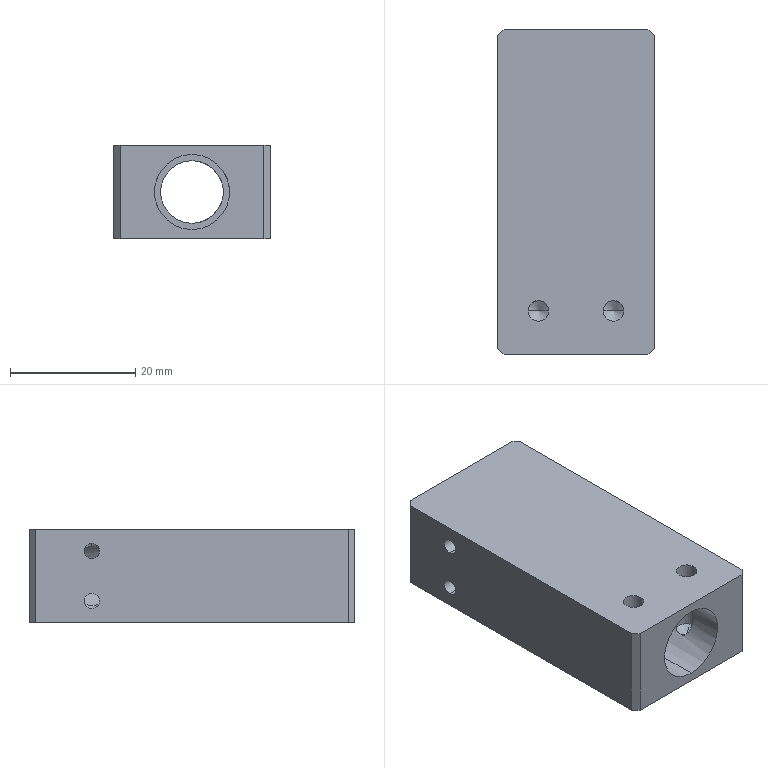Part | NX | features BREP 1 | 1 solid | 37 faces | box 25 x 52 x 15 mm | volume 13996 mm3 | cylinder 18 | plane 12 | cone 7 | commonest cylinder face diameters 3.3 x8 2.5 x4 12 x4 10 x2
STEP:
#1=CARTESIAN_POINT('',(-4.,42.,-5.25));
#2=VERTEX_POINT('',#1);
#3=CARTESIAN_POINT('',(-4.,40.843,-4.472));
#4=VERTEX_POINT('',#3);
#5=CARTESIAN_POINT('',(-4.,42.,-4.));
#6=DIRECTION('',(-1.,0.,0.));
#7=DIRECTION('',(0.,0.,1.));
#8=AXIS2_PLACEMENT_3D('',#5,#6,#7);
#9=CIRCLE('',#8,1.25);
#10=EDGE_CURVE('',#2,#4,#9,.T.);
#11=ORIENTED_EDGE('',*,*,#10,.F.);
#12=CARTESIAN_POINT('',(-12.5,42.,-5.25));
#13=VERTEX_POINT('',#12);
#14=CARTESIAN_POINT('',(-12.5,42.,-5.25));
#15=DIRECTION('',(-1.,0.,0.));
#16=VECTOR('',#15,1000.);
#17=LINE('',#14,#16);
#18=EDGE_CURVE('',#13,#2,#17,.F.);
#19=ORIENTED_EDGE('',*,*,#18,.F.);
#20=CARTESIAN_POINT('',(-12.5,42.,-2.75));
#21=VERTEX_POINT('',#20);
#22=CARTESIAN_POINT('',(-12.5,42.,-4.));
#23=DIRECTION('',(-1.,0.,0.));
#24=DIRECTION('',(0.,0.,1.));
#25=AXIS2_PLACEMENT_3D('',#22,#23,#24);
#26=CIRCLE('',#25,1.25);
#27=EDGE_CURVE('',#13,#21,#26,.T.);
#28=ORIENTED_EDGE('',*,*,#27,.T.);
#29=CARTESIAN_POINT('',(-5.333,42.,-2.75));
#30=VERTEX_POINT('',#29);
#31=CARTESIAN_POINT('',(-12.5,42.,-2.75));
#32=DIRECTION('',(-1.,0.,0.));
#33=VECTOR('',#32,1000.);
#34=LINE('',#31,#33);
#35=EDGE_CURVE('',#21,#30,#34,.F.);
#36=ORIENTED_EDGE('',*,*,#35,.T.);
#37=CARTESIAN_POINT('',(-5.333,42.,-2.75));
#38=CARTESIAN_POINT('',(-5.333,41.765,-2.75));
#39=CARTESIAN_POINT('',(-5.268,41.306,-2.882));
#40=CARTESIAN_POINT('',(-4.954,40.832,-3.412));
#41=CARTESIAN_POINT('',(-4.493,40.719,-3.994));
#42=CARTESIAN_POINT('',(-4.203,40.768,-4.29));
#43=CARTESIAN_POINT('',(-4.,40.843,-4.472));
#44=B_SPLINE_CURVE_WITH_KNOTS('',3,(#37,#38,#39,#40,#41,#42,#43),.UNSPECIFIED.,.F.,.F.,(4,1,1,1,4),(0.,0.25,0.5,0.75,1.),.UNSPECIFIED.);
#45=EDGE_CURVE('',#4,#30,#44,.F.);
#46=ORIENTED_EDGE('',*,*,#45,.F.);
#47=EDGE_LOOP('',(#11,#19,#28,#36,#46));
#48=FACE_BOUND('',#47,.T.);
#49=CARTESIAN_POINT('',(-12.5,42.,-4.));
#50=DIRECTION('',(-1.,0.,0.));
#51=DIRECTION('',(0.,0.,1.));
#52=AXIS2_PLACEMENT_3D('',#49,#50,#51);
#53=CYLINDRICAL_SURFACE('',#52,1.25);
#54=ADVANCED_FACE('',(#48),#53,.F.);
#55=CARTESIAN_POINT('',(-3.689,42.,4.732));
#56=VERTEX_POINT('',#55);
#57=CARTESIAN_POINT('',(-4.,43.157,4.472));
#58=VERTEX_POINT('',#57);
#59=CARTESIAN_POINT('',(-3.689,42.,4.732));
#60=CARTESIAN_POINT('',(-3.689,42.192,4.732));
#61=CARTESIAN_POINT('',(-3.772,42.636,4.668));
#62=CARTESIAN_POINT('',(-3.909,42.961,4.554));
#63=CARTESIAN_POINT('',(-4.,43.157,4.472));
#64=B_SPLINE_CURVE_WITH_KNOTS('',3,(#59,#60,#61,#62,#63),.UNSPECIFIED.,.F.,.F.,(4,1,4),(0.,0.5,1.),.UNSPECIFIED.);
#65=EDGE_CURVE('',#56,#58,#64,.T.);
#66=ORIENTED_EDGE('',*,*,#65,.F.);
#67=CARTESIAN_POINT('',(-4.,42.,5.25));
#68=VERTEX_POINT('',#67);
#69=CARTESIAN_POINT('',(-4.,42.,5.25));
#70=DIRECTION('',(-0.515,0.,0.8572));
#71=VECTOR('',#70,1000.);
#72=LINE('',#69,#71);
#73=EDGE_CURVE('',#56,#68,#72,.T.);
#74=ORIENTED_EDGE('',*,*,#73,.T.);
#75=CARTESIAN_POINT('',(-4.,42.,4.));
#76=DIRECTION('',(-1.,0.,0.));
#77=DIRECTION('',(0.,0.,1.));
#78=AXIS2_PLACEMENT_3D('',#75,#76,#77);
#79=CIRCLE('',#78,1.25);
#80=EDGE_CURVE('',#68,#58,#79,.T.);
#81=ORIENTED_EDGE('',*,*,#80,.T.);
#82=EDGE_LOOP('',(#66,#74,#81));
#83=FACE_BOUND('',#82,.T.);
#84=CARTESIAN_POINT('',(-4.,42.,4.));
#85=DIRECTION('',(-1.,0.,0.));
#86=DIRECTION('',(0.,0.,1.));
#87=AXIS2_PLACEMENT_3D('',#84,#85,#86);
#88=CONICAL_SURFACE('',#87,1.25,1.03);
#89=ADVANCED_FACE('',(#83),#88,.F.);
#90=CARTESIAN_POINT('',(-5.333,42.,2.75));
#91=VERTEX_POINT('',#90);
#92=CARTESIAN_POINT('',(-4.,40.843,4.472));
#93=VERTEX_POINT('',#92);
#94=CARTESIAN_POINT('',(-4.,40.843,4.472));
#95=CARTESIAN_POINT('',(-4.204,40.768,4.29));
#96=CARTESIAN_POINT('',(-4.496,40.719,3.992));
#97=CARTESIAN_POINT('',(-4.954,40.833,3.412));
#98=CARTESIAN_POINT('',(-5.268,41.307,2.882));
#99=CARTESIAN_POINT('',(-5.333,41.765,2.75));
#100=CARTESIAN_POINT('',(-5.333,42.,2.75));
#101=B_SPLINE_CURVE_WITH_KNOTS('',3,(#94,#95,#96,#97,#98,#99,#100),.UNSPECIFIED.,.F.,.F.,(4,1,1,1,4),(0.,0.25,0.5,0.75,1.),.UNSPECIFIED.);
#102=EDGE_CURVE('',#91,#93,#101,.F.);
#103=ORIENTED_EDGE('',*,*,#102,.F.);
#104=CARTESIAN_POINT('',(-12.5,42.,2.75));
#105=VERTEX_POINT('',#104);
#106=CARTESIAN_POINT('',(-12.5,42.,2.75));
#107=DIRECTION('',(-1.,0.,0.));
#108=VECTOR('',#107,1000.);
#109=LINE('',#106,#108);
#110=EDGE_CURVE('',#105,#91,#109,.F.);
#111=ORIENTED_EDGE('',*,*,#110,.F.);
#112=CARTESIAN_POINT('',(-12.5,42.,5.25));
#113=VERTEX_POINT('',#112);
#114=CARTESIAN_POINT('',(-12.5,42.,4.));
#115=DIRECTION('',(-1.,0.,0.));
#116=DIRECTION('',(0.,0.,1.));
#117=AXIS2_PLACEMENT_3D('',#114,#115,#116);
#118=CIRCLE('',#117,1.25);
#119=EDGE_CURVE('',#105,#113,#118,.T.);
#120=ORIENTED_EDGE('',*,*,#119,.T.);
#121=CARTESIAN_POINT('',(-12.5,42.,5.25));
#122=DIRECTION('',(-1.,0.,0.));
#123=VECTOR('',#122,1000.);
#124=LINE('',#121,#123);
#125=EDGE_CURVE('',#113,#68,#124,.F.);
#126=ORIENTED_EDGE('',*,*,#125,.T.);
#127=CARTESIAN_POINT('',(-4.,42.,4.));
#128=DIRECTION('',(-1.,0.,0.));
#129=DIRECTION('',(0.,0.,1.));
#130=AXIS2_PLACEMENT_3D('',#127,#128,#129);
#131=CIRCLE('',#130,1.25);
#132=EDGE_CURVE('',#93,#68,#131,.T.);
#133=ORIENTED_EDGE('',*,*,#132,.F.);
#134=EDGE_LOOP('',(#103,#111,#120,#126,#133));
#135=FACE_BOUND('',#134,.T.);
#136=CARTESIAN_POINT('',(-12.5,42.,4.));
#137=DIRECTION('',(-1.,0.,0.));
#138=DIRECTION('',(0.,0.,1.));
#139=AXIS2_PLACEMENT_3D('',#136,#137,#138);
#140=CYLINDRICAL_SURFACE('',#139,1.25);
#141=ADVANCED_FACE('',(#135),#140,.F.);
#142=CARTESIAN_POINT('',(5.769,47.,1.65));
#143=VERTEX_POINT('',#142);
#144=CARTESIAN_POINT('',(5.769,47.,-1.65));
#145=VERTEX_POINT('',#144);
#146=CARTESIAN_POINT('',(5.769,47.,-1.65));
#147=CARTESIAN_POINT('',(5.769,46.795,-1.65));
#148=CARTESIAN_POINT('',(5.795,46.408,-1.556));
#149=CARTESIAN_POINT('',(5.83,46.152,-1.425));
#150=CARTESIAN_POINT('',(5.886,45.816,-1.179));
#151=CARTESIAN_POINT('',(5.94,45.579,-0.8553));
#152=CARTESIAN_POINT('',(5.966,45.478,-0.6589));
#153=CARTESIAN_POINT('',(5.995,45.365,-0.3068));
#154=CARTESIAN_POINT('',(6.002,45.342,0.0003193));
#155=CARTESIAN_POINT('',(5.995,45.365,0.3073));
#156=CARTESIAN_POINT('',(5.966,45.479,0.6598));
#157=CARTESIAN_POINT('',(5.94,45.58,0.8557));
#158=CARTESIAN_POINT('',(5.886,45.817,1.18));
#159=CARTESIAN_POINT('',(5.83,46.153,1.426));
#160=CARTESIAN_POINT('',(5.794,46.41,1.557));
#161=CARTESIAN_POINT('',(5.769,46.796,1.65));
#162=CARTESIAN_POINT('',(5.769,47.,1.65));
#163=B_SPLINE_CURVE_WITH_KNOTS('',3,(#146,#147,#148,#149,#150,#151,#152,#153,#154,#155,#156,#157,#158,#159,#160,#161,#162),.UNSPECIFIED.,.F.,.F.,(4,1,1,1,1,1,1,1,1,1,1,1,1,1,4),(0.,0.125,0.1875,0.25,0.3125,0.375,0.4375,0.5,0.5625,0.625,0.6875,0.75,0.8125,0.875,1.),.UNSPECIFIED.);
#164=EDGE_CURVE('',#143,#145,#163,.F.);
#165=ORIENTED_EDGE('',*,*,#164,.F.);
#166=CARTESIAN_POINT('',(12.5,47.,1.65));
#167=VERTEX_POINT('',#166);
#168=CARTESIAN_POINT('',(12.5,47.,1.65));
#169=DIRECTION('',(1.,0.,0.));
#170=VECTOR('',#169,1000.);
#171=LINE('',#168,#170);
#172=EDGE_CURVE('',#143,#167,#171,.T.);
#173=ORIENTED_EDGE('',*,*,#172,.T.);
#174=CARTESIAN_POINT('',(12.5,47.,-1.65));
#175=VERTEX_POINT('',#174);
#176=CARTESIAN_POINT('',(12.5,47.,0.));
#177=DIRECTION('',(1.,0.,0.));
#178=DIRECTION('',(0.,0.,-1.));
#179=AXIS2_PLACEMENT_3D('',#176,#177,#178);
#180=CIRCLE('',#179,1.65);
#181=EDGE_CURVE('',#167,#175,#180,.T.);
#182=ORIENTED_EDGE('',*,*,#181,.T.);
#183=CARTESIAN_POINT('',(12.5,47.,-1.65));
#184=DIRECTION('',(1.,0.,0.));
#185=VECTOR('',#184,1000.);
#186=LINE('',#183,#185);
#187=EDGE_CURVE('',#145,#175,#186,.T.);
#188=ORIENTED_EDGE('',*,*,#187,.F.);
#189=EDGE_LOOP('',(#165,#173,#182,#188));
#190=FACE_BOUND('',#189,.T.);
#191=CARTESIAN_POINT('',(12.5,47.,0.));
#192=DIRECTION('',(1.,0.,0.));
#193=DIRECTION('',(0.,0.,-1.));
#194=AXIS2_PLACEMENT_3D('',#191,#192,#193);
#195=CYLINDRICAL_SURFACE('',#194,1.65);
#196=ADVANCED_FACE('',(#190),#195,.F.);
#197=CARTESIAN_POINT('',(4.72,37.,1.65));
#198=VERTEX_POINT('',#197);
#199=CARTESIAN_POINT('',(5.769,37.,1.65));
#200=VERTEX_POINT('',#199);
#201=CARTESIAN_POINT('',(12.5,37.,1.65));
#202=DIRECTION('',(1.,0.,0.));
#203=VECTOR('',#202,1000.);
#204=LINE('',#201,#203);
#205=EDGE_CURVE('',#198,#200,#204,.T.);
#206=ORIENTED_EDGE('',*,*,#205,.T.);
#207=CARTESIAN_POINT('',(12.5,37.,1.65));
#208=VERTEX_POINT('',#207);
#209=CARTESIAN_POINT('',(12.5,37.,1.65));
#210=DIRECTION('',(1.,0.,0.));
#211=VECTOR('',#210,1000.);
#212=LINE('',#209,#211);
#213=EDGE_CURVE('',#200,#208,#212,.T.);
#214=ORIENTED_EDGE('',*,*,#213,.T.);
#215=CARTESIAN_POINT('',(12.5,37.,-1.65));
#216=VERTEX_POINT('',#215);
#217=CARTESIAN_POINT('',(12.5,37.,0.));
#218=DIRECTION('',(1.,0.,0.));
#219=DIRECTION('',(0.,0.,-1.));
#220=AXIS2_PLACEMENT_3D('',#217,#218,#219);
#221=CIRCLE('',#220,1.65);
#222=EDGE_CURVE('',#208,#216,#221,.T.);
#223=ORIENTED_EDGE('',*,*,#222,.T.);
#224=CARTESIAN_POINT('',(5.769,37.,-1.65));
#225=VERTEX_POINT('',#224);
#226=CARTESIAN_POINT('',(12.5,37.,-1.65));
#227=DIRECTION('',(1.,0.,0.));
#228=VECTOR('',#227,1000.);
#229=LINE('',#226,#228);
#230=EDGE_CURVE('',#225,#216,#229,.T.);
#231=ORIENTED_EDGE('',*,*,#230,.F.);
#232=CARTESIAN_POINT('',(4.72,37.,-1.65));
#233=VERTEX_POINT('',#232);
#234=CARTESIAN_POINT('',(12.5,37.,-1.65));
#235=DIRECTION('',(-1.,0.,0.));
#236=VECTOR('',#235,1000.);
#237=LINE('',#234,#236);
#238=EDGE_CURVE('',#225,#233,#237,.T.);
#239=ORIENTED_EDGE('',*,*,#238,.T.);
#240=CARTESIAN_POINT('',(4.72,37.,-1.65));
#241=CARTESIAN_POINT('',(4.72,36.796,-1.65));
#242=CARTESIAN_POINT('',(4.752,36.406,-1.556));
#243=CARTESIAN_POINT('',(4.794,36.154,-1.427));
#244=CARTESIAN_POINT('',(4.863,35.816,-1.179));
#245=CARTESIAN_POINT('',(4.927,35.581,-0.8581));
#246=CARTESIAN_POINT('',(4.959,35.478,-0.6598));
#247=CARTESIAN_POINT('',(4.994,35.365,-0.308));
#248=CARTESIAN_POINT('',(5.003,35.342,-0.0001839));
#249=CARTESIAN_POINT('',(4.994,35.365,0.3075));
#250=CARTESIAN_POINT('',(4.959,35.478,0.6594));
#251=CARTESIAN_POINT('',(4.927,35.581,0.8578));
#252=CARTESIAN_POINT('',(4.863,35.816,1.179));
#253=CARTESIAN_POINT('',(4.794,36.155,1.427));
#254=CARTESIAN_POINT('',(4.752,36.407,1.556));
#255=CARTESIAN_POINT('',(4.72,36.796,1.65));
#256=CARTESIAN_POINT('',(4.72,37.,1.65));
#257=B_SPLINE_CURVE_WITH_KNOTS('',3,(#240,#241,#242,#243,#244,#245,#246,#247,#248,#249,#250,#251,#252,#253,#254,#255,#256),.UNSPECIFIED.,.F.,.F.,(4,1,1,1,1,1,1,1,1,1,1,1,1,1,4),(0.,0.125,0.1875,0.25,0.3125,0.375,0.4375,0.5,0.5625,0.625,0.6875,0.75,0.8125,0.875,1.),.UNSPECIFIED.);
#258=EDGE_CURVE('',#198,#233,#257,.F.);
#259=ORIENTED_EDGE('',*,*,#258,.F.);
#260=EDGE_LOOP('',(#206,#214,#223,#231,#239,#259));
#261=FACE_BOUND('',#260,.T.);
#262=CARTESIAN_POINT('',(12.5,37.,0.));
#263=DIRECTION('',(1.,0.,0.));
#264=DIRECTION('',(0.,0.,-1.));
#265=AXIS2_PLACEMENT_3D('',#262,#263,#264);
#266=CYLINDRICAL_SURFACE('',#265,1.65);
#267=ADVANCED_FACE('',(#261),#266,.F.);
#268=CARTESIAN_POINT('',(-7.65,7.,-4.));
#269=VERTEX_POINT('',#268);
#270=CARTESIAN_POINT('',(-4.472,6.377,-4.));
#271=VERTEX_POINT('',#270);
#272=CARTESIAN_POINT('',(-6.,7.,-4.));
#273=DIRECTION('',(0.,0.,1.));
#274=DIRECTION('',(1.,0.,0.));
#275=AXIS2_PLACEMENT_3D('',#272,#273,#274);
#276=CIRCLE('',#275,1.65);
#277=EDGE_CURVE('',#269,#271,#276,.T.);
#278=ORIENTED_EDGE('',*,*,#277,.F.);
#279=CARTESIAN_POINT('',(-7.65,7.,7.5));
#280=VERTEX_POINT('',#279);
#281=CARTESIAN_POINT('',(-7.65,7.,7.5));
#282=DIRECTION('',(0.,0.,1.));
#283=VECTOR('',#282,1000.);
#284=LINE('',#281,#283);
#285=EDGE_CURVE('',#280,#269,#284,.F.);
#286=ORIENTED_EDGE('',*,*,#285,.F.);
#287=CARTESIAN_POINT('',(-4.35,7.,7.5));
#288=VERTEX_POINT('',#287);
#289=CARTESIAN_POINT('',(-6.,7.,7.5));
#290=DIRECTION('',(0.,0.,1.));
#291=DIRECTION('',(1.,0.,0.));
#292=AXIS2_PLACEMENT_3D('',#289,#290,#291);
#293=CIRCLE('',#292,1.65);
#294=EDGE_CURVE('',#280,#288,#293,.T.);
#295=ORIENTED_EDGE('',*,*,#294,.T.);
#296=CARTESIAN_POINT('',(-4.35,7.,4.132));
#297=VERTEX_POINT('',#296);
#298=CARTESIAN_POINT('',(-4.35,7.,7.5));
#299=DIRECTION('',(0.,0.,1.));
#300=VECTOR('',#299,1000.);
#301=LINE('',#298,#300);
#302=EDGE_CURVE('',#288,#297,#301,.F.);
#303=ORIENTED_EDGE('',*,*,#302,.T.);
#304=CARTESIAN_POINT('',(-4.35,7.,4.132));
#305=CARTESIAN_POINT('',(-4.35,6.798,4.132));
#306=CARTESIAN_POINT('',(-4.418,6.41,4.068));
#307=CARTESIAN_POINT('',(-4.74,5.897,3.689));
#308=CARTESIAN_POINT('',(-5.028,5.65,3.294));
#309=CARTESIAN_POINT('',(-5.371,5.462,2.699));
#310=CARTESIAN_POINT('',(-5.603,5.394,2.175));
#311=CARTESIAN_POINT('',(-5.809,5.358,1.552));
#312=CARTESIAN_POINT('',(-5.936,5.351,0.935));
#313=CARTESIAN_POINT('',(-5.989,5.35,0.4749));
#314=CARTESIAN_POINT('',(-6.006,5.35,-0.06688));
#315=CARTESIAN_POINT('',(-5.98,5.35,-0.5238));
#316=CARTESIAN_POINT('',(-5.96,5.35,-0.6899));
#317=CARTESIAN_POINT('',(-5.925,5.351,-0.9759));
#318=CARTESIAN_POINT('',(-5.807,5.359,-1.559));
#319=CARTESIAN_POINT('',(-5.63,5.386,-2.106));
#320=CARTESIAN_POINT('',(-5.353,5.474,-2.735));
#321=CARTESIAN_POINT('',(-5.084,5.608,-3.203));
#322=CARTESIAN_POINT('',(-4.711,5.928,-3.731));
#323=CARTESIAN_POINT('',(-4.539,6.214,-3.926));
#324=CARTESIAN_POINT('',(-4.472,6.377,-4.));
#325=B_SPLINE_CURVE_WITH_KNOTS('',3,(#304,#305,#306,#307,#308,#309,#310,#311,#312,#313,#314,#315,#316,#317,#318,#319,#320,#321,#322,#323,#324),.UNSPECIFIED.,.F.,.F.,(4,1,1,1,1,1,1,1,1,1,1,1,1,1,1,1,1,1,4),(0.,0.0625,0.125,0.1875,0.25,0.3125,0.375,0.4375,0.5,0.5312,0.5625,0.5938,0.625,0.6875,0.75,0.8125,0.875,0.9375,1.),.UNSPECIFIED.);
#326=EDGE_CURVE('',#271,#297,#325,.F.);
#327=ORIENTED_EDGE('',*,*,#326,.F.);
#328=EDGE_LOOP('',(#278,#286,#295,#303,#327));
#329=FACE_BOUND('',#328,.T.);
#330=CARTESIAN_POINT('',(-6.,7.,7.5));
#331=DIRECTION('',(0.,0.,1.));
#332=DIRECTION('',(1.,0.,0.));
#333=AXIS2_PLACEMENT_3D('',#330,#331,#332);
#334=CYLINDRICAL_SURFACE('',#333,1.65);
#335=ADVANCED_FACE('',(#329),#334,.F.);
#336=CARTESIAN_POINT('',(-4.429,7.,-4.048));
#337=VERTEX_POINT('',#336);
#338=CARTESIAN_POINT('',(-6.,7.,-4.991));
#339=VERTEX_POINT('',#338);
#340=CARTESIAN_POINT('',(-4.35,7.,-4.));
#341=DIRECTION('',(0.8572,0.,0.515));
#342=VECTOR('',#341,1000.);
#343=LINE('',#340,#342);
#344=EDGE_CURVE('',#337,#339,#343,.F.);
#345=ORIENTED_EDGE('',*,*,#344,.T.);
#346=CARTESIAN_POINT('',(-7.65,7.,-4.));
#347=DIRECTION('',(-0.8572,0.,0.515));
#348=VECTOR('',#347,1000.);
#349=LINE('',#346,#348);
#350=EDGE_CURVE('',#269,#339,#349,.F.);
#351=ORIENTED_EDGE('',*,*,#350,.F.);
#352=ORIENTED_EDGE('',*,*,#277,.T.);
#353=CARTESIAN_POINT('',(-4.429,7.,-4.048));
#354=CARTESIAN_POINT('',(-4.429,6.794,-4.047));
#355=CARTESIAN_POINT('',(-4.444,6.586,-4.032));
#356=CARTESIAN_POINT('',(-4.472,6.377,-4.));
#357=B_SPLINE_CURVE_WITH_KNOTS('',3,(#353,#354,#355,#356),.UNSPECIFIED.,.F.,.F.,(4,4),(0.,1.),.UNSPECIFIED.);
#358=EDGE_CURVE('',#337,#271,#357,.T.);
#359=ORIENTED_EDGE('',*,*,#358,.F.);
#360=EDGE_LOOP('',(#345,#351,#352,#359));
#361=FACE_BOUND('',#360,.T.);
#362=CARTESIAN_POINT('',(-6.,7.,-4.));
#363=DIRECTION('',(0.,0.,1.));
#364=DIRECTION('',(1.,0.,0.));
#365=AXIS2_PLACEMENT_3D('',#362,#363,#364);
#366=CONICAL_SURFACE('',#365,1.65,1.03);
#367=ADVANCED_FACE('',(#361),#366,.F.);
#368=CARTESIAN_POINT('',(4.35,7.,4.132));
#369=VERTEX_POINT('',#368);
#370=CARTESIAN_POINT('',(4.472,6.377,-4.));
#371=VERTEX_POINT('',#370);
#372=CARTESIAN_POINT('',(4.472,6.377,-4.));
#373=CARTESIAN_POINT('',(4.538,6.214,-3.926));
#374=CARTESIAN_POINT('',(4.711,5.928,-3.732));
#375=CARTESIAN_POINT('',(5.083,5.609,-3.205));
#376=CARTESIAN_POINT('',(5.353,5.474,-2.736));
#377=CARTESIAN_POINT('',(5.63,5.386,-2.106));
#378=CARTESIAN_POINT('',(5.807,5.359,-1.559));
#379=CARTESIAN_POINT('',(5.926,5.351,-0.9746));
#380=CARTESIAN_POINT('',(5.96,5.35,-0.6898));
#381=CARTESIAN_POINT('',(5.98,5.35,-0.524));
#382=CARTESIAN_POINT('',(6.006,5.35,-0.06823));
#383=CARTESIAN_POINT('',(5.989,5.35,0.4722));
#384=CARTESIAN_POINT('',(5.936,5.351,0.9341));
#385=CARTESIAN_POINT('',(5.808,5.358,1.553));
#386=CARTESIAN_POINT('',(5.603,5.394,2.175));
#387=CARTESIAN_POINT('',(5.371,5.462,2.699));
#388=CARTESIAN_POINT('',(5.029,5.65,3.293));
#389=CARTESIAN_POINT('',(4.742,5.895,3.686));
#390=CARTESIAN_POINT('',(4.418,6.409,4.068));
#391=CARTESIAN_POINT('',(4.35,6.797,4.132));
#392=CARTESIAN_POINT('',(4.35,7.,4.132));
#393=B_SPLINE_CURVE_WITH_KNOTS('',3,(#372,#373,#374,#375,#376,#377,#378,#379,#380,#381,#382,#383,#384,#385,#386,#387,#388,#389,#390,#391,#392),.UNSPECIFIED.,.F.,.F.,(4,1,1,1,1,1,1,1,1,1,1,1,1,1,1,1,1,1,4),(0.,0.0625,0.125,0.1875,0.25,0.3125,0.375,0.4062,0.4375,0.4688,0.5,0.5625,0.625,0.6875,0.75,0.8125,0.875,0.9375,1.),.UNSPECIFIED.);
#394=EDGE_CURVE('',#369,#371,#393,.F.);
#395=ORIENTED_EDGE('',*,*,#394,.F.);
#396=CARTESIAN_POINT('',(4.35,7.,7.5));
#397=VERTEX_POINT('',#396);
#398=CARTESIAN_POINT('',(4.35,7.,7.5));
#399=DIRECTION('',(0.,0.,1.));
#400=VECTOR('',#399,1000.);
#401=LINE('',#398,#400);
#402=EDGE_CURVE('',#397,#369,#401,.F.);
#403=ORIENTED_EDGE('',*,*,#402,.F.);
#404=CARTESIAN_POINT('',(7.65,7.,7.5));
#405=VERTEX_POINT('',#404);
#406=CARTESIAN_POINT('',(6.,7.,7.5));
#407=DIRECTION('',(0.,0.,1.));
#408=DIRECTION('',(1.,0.,0.));
#409=AXIS2_PLACEMENT_3D('',#406,#407,#408);
#410=CIRCLE('',#409,1.65);
#411=EDGE_CURVE('',#397,#405,#410,.T.);
#412=ORIENTED_EDGE('',*,*,#411,.T.);
#413=CARTESIAN_POINT('',(7.65,7.,-4.));
#414=VERTEX_POINT('',#413);
#415=CARTESIAN_POINT('',(7.65,7.,7.5));
#416=DIRECTION('',(0.,0.,1.));
#417=VECTOR('',#416,1000.);
#418=LINE('',#415,#417);
#419=EDGE_CURVE('',#405,#414,#418,.F.);
#420=ORIENTED_EDGE('',*,*,#419,.T.);
#421=CARTESIAN_POINT('',(6.,7.,-4.));
#422=DIRECTION('',(0.,0.,1.));
#423=DIRECTION('',(1.,0.,0.));
#424=AXIS2_PLACEMENT_3D('',#421,#422,#423);
#425=CIRCLE('',#424,1.65);
#426=EDGE_CURVE('',#371,#414,#425,.T.);
#427=ORIENTED_EDGE('',*,*,#426,.F.);
#428=EDGE_LOOP('',(#395,#403,#412,#420,#427));
#429=FACE_BOUND('',#428,.T.);
#430=CARTESIAN_POINT('',(6.,7.,7.5));
#431=DIRECTION('',(0.,0.,1.));
#432=DIRECTION('',(1.,0.,0.));
#433=AXIS2_PLACEMENT_3D('',#430,#431,#432);
#434=CYLINDRICAL_SURFACE('',#433,1.65);
#435=ADVANCED_FACE('',(#429),#434,.F.);
#436=CARTESIAN_POINT('',(6.,7.,-4.991));
#437=VERTEX_POINT('',#436);
#438=CARTESIAN_POINT('',(7.65,7.,-4.));
#439=DIRECTION('',(0.8572,0.,0.515));
#440=VECTOR('',#439,1000.);
#441=LINE('',#438,#440);
#442=EDGE_CURVE('',#414,#437,#441,.F.);
#443=ORIENTED_EDGE('',*,*,#442,.T.);
#444=CARTESIAN_POINT('',(4.429,7.,-4.048));
#445=VERTEX_POINT('',#444);
#446=CARTESIAN_POINT('',(4.35,7.,-4.));
#447=DIRECTION('',(-0.8572,0.,0.515));
#448=VECTOR('',#447,1000.);
#449=LINE('',#446,#448);
#450=EDGE_CURVE('',#445,#437,#449,.F.);
#451=ORIENTED_EDGE('',*,*,#450,.F.);
#452=CARTESIAN_POINT('',(4.472,6.377,-4.));
#453=CARTESIAN_POINT('',(4.444,6.586,-4.032));
#454=CARTESIAN_POINT('',(4.429,6.794,-4.047));
#455=CARTESIAN_POINT('',(4.429,7.,-4.048));
#456=B_SPLINE_CURVE_WITH_KNOTS('',3,(#452,#453,#454,#455),.UNSPECIFIED.,.F.,.F.,(4,4),(0.,1.),.UNSPECIFIED.);
#457=EDGE_CURVE('',#371,#445,#456,.T.);
#458=ORIENTED_EDGE('',*,*,#457,.F.);
#459=ORIENTED_EDGE('',*,*,#426,.T.);
#460=EDGE_LOOP('',(#443,#451,#458,#459));
#461=FACE_BOUND('',#460,.T.);
#462=CARTESIAN_POINT('',(6.,7.,-4.));
#463=DIRECTION('',(0.,0.,1.));
#464=DIRECTION('',(1.,0.,0.));
#465=AXIS2_PLACEMENT_3D('',#462,#463,#464);
#466=CONICAL_SURFACE('',#465,1.65,1.03);
#467=ADVANCED_FACE('',(#461),#466,.F.);
#468=CARTESIAN_POINT('',(0.,15.,5.));
#469=VERTEX_POINT('',#468);
#470=CARTESIAN_POINT('',(0.,15.,-5.));
#471=VERTEX_POINT('',#470);
#472=CARTESIAN_POINT('',(0.,15.,0.));
#473=DIRECTION('',(0.,-1.,0.));
#474=DIRECTION('',(0.,0.,-1.));
#475=AXIS2_PLACEMENT_3D('',#472,#473,#474);
#476=CIRCLE('',#475,5.);
#477=EDGE_CURVE('',#469,#471,#476,.T.);
#478=ORIENTED_EDGE('',*,*,#477,.T.);
#479=CARTESIAN_POINT('',(0.,37.,-5.));
#480=VERTEX_POINT('',#479);
#481=CARTESIAN_POINT('',(0.,0.,-5.));
#482=DIRECTION('',(0.,1.,0.));
#483=VECTOR('',#482,1000.);
#484=LINE('',#481,#483);
#485=EDGE_CURVE('',#480,#471,#484,.F.);
#486=ORIENTED_EDGE('',*,*,#485,.F.);
#487=CARTESIAN_POINT('',(0.,37.,5.));
#488=VERTEX_POINT('',#487);
#489=CARTESIAN_POINT('',(0.,37.,0.));
#490=DIRECTION('',(0.,1.,0.));
#491=DIRECTION('',(0.,0.,1.));
#492=AXIS2_PLACEMENT_3D('',#489,#490,#491);
#493=CIRCLE('',#492,5.);
#494=EDGE_CURVE('',#480,#488,#493,.T.);
#495=ORIENTED_EDGE('',*,*,#494,.T.);
#496=CARTESIAN_POINT('',(0.,0.,5.));
#497=DIRECTION('',(0.,1.,0.));
#498=VECTOR('',#497,1000.);
#499=LINE('',#496,#498);
#500=EDGE_CURVE('',#488,#469,#499,.F.);
#501=ORIENTED_EDGE('',*,*,#500,.T.);
#502=EDGE_LOOP('',(#478,#486,#495,#501));
#503=FACE_BOUND('',#502,.T.);
#504=CARTESIAN_POINT('',(0.,0.,0.));
#505=DIRECTION('',(0.,1.,0.));
#506=DIRECTION('',(0.,0.,1.));
#507=AXIS2_PLACEMENT_3D('',#504,#505,#506);
#508=CYLINDRICAL_SURFACE('',#507,5.);
#509=ADVANCED_FACE('',(#503),#508,.F.);
#510=CARTESIAN_POINT('',(0.,15.,6.));
#511=VERTEX_POINT('',#510);
#512=CARTESIAN_POINT('',(0.,15.,-6.));
#513=VERTEX_POINT('',#512);
#514=CARTESIAN_POINT('',(0.,15.,0.));
#515=DIRECTION('',(0.,-1.,0.));
#516=DIRECTION('',(0.,0.,-1.));
#517=AXIS2_PLACEMENT_3D('',#514,#515,#516);
#518=CIRCLE('',#517,6.);
#519=EDGE_CURVE('',#511,#513,#518,.T.);
#520=ORIENTED_EDGE('',*,*,#519,.F.);
#521=CARTESIAN_POINT('',(0.,0.,6.));
#522=VERTEX_POINT('',#521);
#523=CARTESIAN_POINT('',(0.,15.,6.));
#524=DIRECTION('',(0.,-1.,0.));
#525=VECTOR('',#524,1000.);
#526=LINE('',#523,#525);
#527=EDGE_CURVE('',#511,#522,#526,.T.);
#528=ORIENTED_EDGE('',*,*,#527,.T.);
#529=CARTESIAN_POINT('',(0.,0.,-6.));
#530=VERTEX_POINT('',#529);
#531=CARTESIAN_POINT('',(0.,0.,0.));
#532=DIRECTION('',(0.,-1.,0.));
#533=DIRECTION('',(0.,0.,-1.));
#534=AXIS2_PLACEMENT_3D('',#531,#532,#533);
#535=CIRCLE('',#534,6.);
#536=EDGE_CURVE('',#522,#530,#535,.T.);
#537=ORIENTED_EDGE('',*,*,#536,.T.);
#538=CARTESIAN_POINT('',(0.,15.,-6.));
#539=DIRECTION('',(0.,-1.,0.));
#540=VECTOR('',#539,1000.);
#541=LINE('',#538,#540);
#542=EDGE_CURVE('',#513,#530,#541,.T.);
#543=ORIENTED_EDGE('',*,*,#542,.F.);
#544=EDGE_LOOP('',(#520,#528,#537,#543));
#545=FACE_BOUND('',#544,.T.);
#546=ORIENTED_EDGE('',*,*,#326,.T.);
#547=CARTESIAN_POINT('',(-4.472,7.623,-4.));
#548=VERTEX_POINT('',#547);
#549=CARTESIAN_POINT('',(-4.35,7.,4.132));
#550=CARTESIAN_POINT('',(-4.35,7.42,4.132));
#551=CARTESIAN_POINT('',(-4.645,8.02,3.816));
#552=CARTESIAN_POINT('',(-5.014,8.34,3.316));
#553=CARTESIAN_POINT('',(-5.382,8.543,2.678));
#554=CARTESIAN_POINT('',(-5.542,8.586,2.31));
#555=CARTESIAN_POINT('',(-5.692,8.622,1.913));
#556=CARTESIAN_POINT('',(-5.809,8.64,1.511));
#557=CARTESIAN_POINT('',(-5.845,8.642,1.361));
#558=CARTESIAN_POINT('',(-5.928,8.649,0.9698));
#559=CARTESIAN_POINT('',(-5.994,8.65,0.4975));
#560=CARTESIAN_POINT('',(-6.003,8.65,-0.1446));
#561=CARTESIAN_POINT('',(-5.983,8.65,-0.483));
#562=CARTESIAN_POINT('',(-5.95,8.649,-0.7774));
#563=CARTESIAN_POINT('',(-5.941,8.649,-0.8561));
#564=CARTESIAN_POINT('',(-5.86,8.644,-1.31));
#565=CARTESIAN_POINT('',(-5.784,8.636,-1.604));
#566=CARTESIAN_POINT('',(-5.692,8.621,-1.901));
#567=CARTESIAN_POINT('',(-5.627,8.609,-2.089));
#568=CARTESIAN_POINT('',(-5.478,8.568,-2.459));
#569=CARTESIAN_POINT('',(-5.292,8.494,-2.837));
#570=CARTESIAN_POINT('',(-5.091,8.396,-3.195));
#571=CARTESIAN_POINT('',(-4.701,8.063,-3.743));
#572=CARTESIAN_POINT('',(-4.538,7.784,-3.927));
#573=CARTESIAN_POINT('',(-4.472,7.623,-4.));
#574=B_SPLINE_CURVE_WITH_KNOTS('',3,(#549,#550,#551,#552,#553,#554,#555,#556,#557,#558,#559,#560,#561,#562,#563,#564,#565,#566,#567,#568,#569,#570,#571,#572,#573),.UNSPECIFIED.,.F.,.F.,(4,1,1,1,1,1,1,1,1,1,1,1,1,1,1,1,1,1,1,1,1,1,4),(0.,0.125,0.1875,0.25,0.3125,0.3438,0.375,0.4062,0.4375,0.5,0.5312,0.5625,0.5938,0.625,0.6562,0.6875,0.7188,0.75,0.7812,0.8125,0.875,0.9375,1.),.UNSPECIFIED.);
#575=EDGE_CURVE('',#297,#548,#574,.T.);
#576=ORIENTED_EDGE('',*,*,#575,.T.);
#577=CARTESIAN_POINT('',(-4.472,7.623,-4.));
#578=CARTESIAN_POINT('',(-4.444,7.414,-4.032));
#579=CARTESIAN_POINT('',(-4.429,7.206,-4.047));
#580=CARTESIAN_POINT('',(-4.429,7.,-4.048));
#581=B_SPLINE_CURVE_WITH_KNOTS('',3,(#577,#578,#579,#580),.UNSPECIFIED.,.F.,.F.,(4,4),(0.,1.),.UNSPECIFIED.);
#582=EDGE_CURVE('',#548,#337,#581,.T.);
#583=ORIENTED_EDGE('',*,*,#582,.T.);
#584=ORIENTED_EDGE('',*,*,#358,.T.);
#585=EDGE_LOOP('',(#546,#576,#583,#584));
#586=FACE_BOUND('',#585,.T.);
#587=CARTESIAN_POINT('',(0.,15.,0.));
#588=DIRECTION('',(0.,-1.,0.));
#589=DIRECTION('',(0.,0.,-1.));
#590=AXIS2_PLACEMENT_3D('',#587,#588,#589);
#591=CYLINDRICAL_SURFACE('',#590,6.);
#592=ADVANCED_FACE('',(#545,#586),#591,.F.);
#593=CARTESIAN_POINT('',(0.,37.,-6.));
#594=VERTEX_POINT('',#593);
#595=CARTESIAN_POINT('',(0.,37.,6.));
#596=VERTEX_POINT('',#595);
#597=CARTESIAN_POINT('',(0.,37.,0.));
#598=DIRECTION('',(0.,1.,0.));
#599=DIRECTION('',(0.,0.,1.));
#600=AXIS2_PLACEMENT_3D('',#597,#598,#599);
#601=CIRCLE('',#600,6.);
#602=EDGE_CURVE('',#594,#596,#601,.T.);
#603=ORIENTED_EDGE('',*,*,#602,.F.);
#604=CARTESIAN_POINT('',(0.,52.,-6.));
#605=VERTEX_POINT('',#604);
#606=CARTESIAN_POINT('',(0.,37.,-6.));
#607=DIRECTION('',(0.,1.,0.));
#608=VECTOR('',#607,1000.);
#609=LINE('',#606,#608);
#610=EDGE_CURVE('',#605,#594,#609,.F.);
#611=ORIENTED_EDGE('',*,*,#610,.F.);
#612=CARTESIAN_POINT('',(0.,52.,6.));
#613=VERTEX_POINT('',#612);
#614=CARTESIAN_POINT('',(0.,52.,0.));
#615=DIRECTION('',(0.,1.,0.));
#616=DIRECTION('',(0.,0.,1.));
#617=AXIS2_PLACEMENT_3D('',#614,#615,#616);
#618=CIRCLE('',#617,6.);
#619=EDGE_CURVE('',#605,#613,#618,.T.);
#620=ORIENTED_EDGE('',*,*,#619,.T.);
#621=CARTESIAN_POINT('',(0.,37.,6.));
#622=DIRECTION('',(0.,1.,0.));
#623=VECTOR('',#622,1000.);
#624=LINE('',#621,#623);
#625=EDGE_CURVE('',#613,#596,#624,.F.);
#626=ORIENTED_EDGE('',*,*,#625,.T.);
#627=EDGE_LOOP('',(#603,#611,#620,#626));
#628=FACE_BOUND('',#627,.T.);
#629=CARTESIAN_POINT('',(-4.,40.843,4.472));
#630=CARTESIAN_POINT('',(-3.909,41.039,4.553));
#631=CARTESIAN_POINT('',(-3.772,41.364,4.668));
#632=CARTESIAN_POINT('',(-3.689,41.808,4.732));
#633=CARTESIAN_POINT('',(-3.689,42.,4.732));
#634=B_SPLINE_CURVE_WITH_KNOTS('',3,(#629,#630,#631,#632,#633),.UNSPECIFIED.,.F.,.F.,(4,1,4),(0.,0.5,1.),.UNSPECIFIED.);
#635=EDGE_CURVE('',#93,#56,#634,.T.);
#636=ORIENTED_EDGE('',*,*,#635,.T.);
#637=ORIENTED_EDGE('',*,*,#65,.T.);
#638=CARTESIAN_POINT('',(-4.,43.157,4.472));
#639=CARTESIAN_POINT('',(-4.359,43.288,4.151));
#640=CARTESIAN_POINT('',(-5.013,43.325,3.39));
#641=CARTESIAN_POINT('',(-5.332,42.491,2.75));
#642=CARTESIAN_POINT('',(-5.333,42.,2.75));
#643=B_SPLINE_CURVE_WITH_KNOTS('',3,(#638,#639,#640,#641,#642),.UNSPECIFIED.,.F.,.F.,(4,1,4),(0.,0.5,1.),.UNSPECIFIED.);
#644=EDGE_CURVE('',#58,#91,#643,.T.);
#645=ORIENTED_EDGE('',*,*,#644,.T.);
#646=ORIENTED_EDGE('',*,*,#102,.T.);
#647=EDGE_LOOP('',(#636,#637,#645,#646));
#648=FACE_BOUND('',#647,.T.);
#649=CARTESIAN_POINT('',(-4.,43.157,-4.472));
#650=VERTEX_POINT('',#649);
#651=CARTESIAN_POINT('',(-4.,43.157,-4.472));
#652=CARTESIAN_POINT('',(-3.909,42.961,-4.554));
#653=CARTESIAN_POINT('',(-3.772,42.627,-4.668));
#654=CARTESIAN_POINT('',(-3.647,42.,-4.764));
#655=CARTESIAN_POINT('',(-3.772,41.372,-4.668));
#656=CARTESIAN_POINT('',(-3.909,41.039,-4.553));
#657=CARTESIAN_POINT('',(-4.,40.843,-4.472));
#658=B_SPLINE_CURVE_WITH_KNOTS('',3,(#651,#652,#653,#654,#655,#656,#657),.UNSPECIFIED.,.F.,.F.,(4,1,1,1,4),(0.,0.25,0.5,0.75,1.),.UNSPECIFIED.);
#659=EDGE_CURVE('',#650,#4,#658,.T.);
#660=ORIENTED_EDGE('',*,*,#659,.T.);
#661=ORIENTED_EDGE('',*,*,#45,.T.);
#662=CARTESIAN_POINT('',(-5.333,42.,-2.75));
#663=CARTESIAN_POINT('',(-5.332,42.476,-2.75));
#664=CARTESIAN_POINT('',(-5.013,43.332,-3.39));
#665=CARTESIAN_POINT('',(-4.36,43.289,-4.15));
#666=CARTESIAN_POINT('',(-4.,43.157,-4.472));
#667=B_SPLINE_CURVE_WITH_KNOTS('',3,(#662,#663,#664,#665,#666),.UNSPECIFIED.,.F.,.F.,(4,1,4),(0.,0.5,1.),.UNSPECIFIED.);
#668=EDGE_CURVE('',#30,#650,#667,.T.);
#669=ORIENTED_EDGE('',*,*,#668,.T.);
#670=EDGE_LOOP('',(#660,#661,#669));
#671=FACE_BOUND('',#670,.T.);
#672=CARTESIAN_POINT('',(0.,37.,0.));
#673=DIRECTION('',(0.,1.,0.));
#674=DIRECTION('',(0.,0.,1.));
#675=AXIS2_PLACEMENT_3D('',#672,#673,#674);
#676=CYLINDRICAL_SURFACE('',#675,6.);
#677=ADVANCED_FACE('',(#628,#648,#671),#676,.F.);
#678=CARTESIAN_POINT('',(-12.5,51.,-7.5));
#679=VERTEX_POINT('',#678);
#680=CARTESIAN_POINT('',(-12.5,1.,-7.5));
#681=VERTEX_POINT('',#680);
#682=CARTESIAN_POINT('',(-12.5,52.,-7.5));
#683=DIRECTION('',(0.,-1.,0.));
#684=VECTOR('',#683,1000.);
#685=LINE('',#682,#684);
#686=EDGE_CURVE('',#679,#681,#685,.T.);
#687=ORIENTED_EDGE('',*,*,#686,.T.);
#688=CARTESIAN_POINT('',(-12.5,1.,7.5));
#689=VERTEX_POINT('',#688);
#690=CARTESIAN_POINT('',(-12.5,1.,-7.5));
#691=DIRECTION('',(0.,0.,1.));
#692=VECTOR('',#691,1000.);
#693=LINE('',#690,#692);
#694=EDGE_CURVE('',#681,#689,#693,.T.);
#695=ORIENTED_EDGE('',*,*,#694,.T.);
#696=CARTESIAN_POINT('',(-12.5,51.,7.5));
#697=VERTEX_POINT('',#696);
#698=CARTESIAN_POINT('',(-12.5,52.,7.5));
#699=DIRECTION('',(0.,-1.,0.));
#700=VECTOR('',#699,1000.);
#701=LINE('',#698,#700);
#702=EDGE_CURVE('',#697,#689,#701,.T.);
#703=ORIENTED_EDGE('',*,*,#702,.F.);
#704=CARTESIAN_POINT('',(-12.5,51.,-7.5));
#705=DIRECTION('',(0.,0.,-1.));
#706=VECTOR('',#705,1000.);
#707=LINE('',#704,#706);
#708=EDGE_CURVE('',#697,#679,#707,.T.);
#709=ORIENTED_EDGE('',*,*,#708,.T.);
#710=EDGE_LOOP('',(#687,#695,#703,#709));
#711=FACE_BOUND('',#710,.T.);
#712=CARTESIAN_POINT('',(-12.5,42.,-4.));
#713=DIRECTION('',(-1.,0.,0.));
#714=DIRECTION('',(0.,0.,1.));
#715=AXIS2_PLACEMENT_3D('',#712,#713,#714);
#716=CIRCLE('',#715,1.25);
#717=EDGE_CURVE('',#21,#13,#716,.T.);
#718=ORIENTED_EDGE('',*,*,#717,.F.);
#719=ORIENTED_EDGE('',*,*,#27,.F.);
#720=EDGE_LOOP('',(#718,#719));
#721=FACE_BOUND('',#720,.T.);
#722=CARTESIAN_POINT('',(-12.5,42.,4.));
#723=DIRECTION('',(-1.,0.,0.));
#724=DIRECTION('',(0.,0.,1.));
#725=AXIS2_PLACEMENT_3D('',#722,#723,#724);
#726=CIRCLE('',#725,1.25);
#727=EDGE_CURVE('',#113,#105,#726,.T.);
#728=ORIENTED_EDGE('',*,*,#727,.F.);
#729=ORIENTED_EDGE('',*,*,#119,.F.);
#730=EDGE_LOOP('',(#728,#729));
#731=FACE_BOUND('',#730,.T.);
#732=CARTESIAN_POINT('',(-12.5,52.,-7.5));
#733=DIRECTION('',(1.,0.,0.));
#734=DIRECTION('',(0.,1.,0.));
#735=AXIS2_PLACEMENT_3D('',#732,#733,#734);
#736=PLANE('',#735);
#737=ADVANCED_FACE('',(#711,#721,#731),#736,.F.);
#738=CARTESIAN_POINT('',(-11.5,0.,7.5));
#739=VERTEX_POINT('',#738);
#740=CARTESIAN_POINT('',(11.5,0.,7.5));
#741=VERTEX_POINT('',#740);
#742=CARTESIAN_POINT('',(-12.5,0.,7.5));
#743=DIRECTION('',(1.,0.,0.));
#744=VECTOR('',#743,1000.);
#745=LINE('',#742,#744);
#746=EDGE_CURVE('',#739,#741,#745,.T.);
#747=ORIENTED_EDGE('',*,*,#746,.T.);
#748=CARTESIAN_POINT('',(12.5,1.,7.5));
#749=VERTEX_POINT('',#748);
#750=CARTESIAN_POINT('',(12.5,1.,7.5));
#751=DIRECTION('',(0.7071,0.7071,0.));
#752=VECTOR('',#751,1000.);
#753=LINE('',#750,#752);
#754=EDGE_CURVE('',#741,#749,#753,.T.);
#755=ORIENTED_EDGE('',*,*,#754,.T.);
#756=CARTESIAN_POINT('',(12.5,51.,7.5));
#757=VERTEX_POINT('',#756);
#758=CARTESIAN_POINT('',(12.5,52.,7.5));
#759=DIRECTION('',(0.,-1.,0.));
#760=VECTOR('',#759,1000.);
#761=LINE('',#758,#760);
#762=EDGE_CURVE('',#757,#749,#761,.T.);
#763=ORIENTED_EDGE('',*,*,#762,.F.);
#764=CARTESIAN_POINT('',(11.5,52.,7.5));
#765=VERTEX_POINT('',#764);
#766=CARTESIAN_POINT('',(11.5,52.,7.5));
#767=DIRECTION('',(-0.7071,0.7071,0.));
#768=VECTOR('',#767,1000.);
#769=LINE('',#766,#768);
#770=EDGE_CURVE('',#757,#765,#769,.T.);
#771=ORIENTED_EDGE('',*,*,#770,.T.);
#772=CARTESIAN_POINT('',(-11.5,52.,7.5));
#773=VERTEX_POINT('',#772);
#774=CARTESIAN_POINT('',(-12.5,52.,7.5));
#775=DIRECTION('',(1.,0.,0.));
#776=VECTOR('',#775,1000.);
#777=LINE('',#774,#776);
#778=EDGE_CURVE('',#773,#765,#777,.T.);
#779=ORIENTED_EDGE('',*,*,#778,.F.);
#780=CARTESIAN_POINT('',(-11.5,52.,7.5));
#781=DIRECTION('',(-0.7071,-0.7071,0.));
#782=VECTOR('',#781,1000.);
#783=LINE('',#780,#782);
#784=EDGE_CURVE('',#773,#697,#783,.T.);
#785=ORIENTED_EDGE('',*,*,#784,.T.);
#786=ORIENTED_EDGE('',*,*,#702,.T.);
#787=CARTESIAN_POINT('',(-12.5,1.,7.5));
#788=DIRECTION('',(0.7071,-0.7071,0.));
#789=VECTOR('',#788,1000.);
#790=LINE('',#787,#789);
#791=EDGE_CURVE('',#689,#739,#790,.T.);
#792=ORIENTED_EDGE('',*,*,#791,.T.);
#793=EDGE_LOOP('',(#747,#755,#763,#771,#779,#785,#786,#792));
#794=FACE_BOUND('',#793,.T.);
#795=CARTESIAN_POINT('',(-6.,7.,7.5));
#796=DIRECTION('',(0.,0.,1.));
#797=DIRECTION('',(1.,0.,0.));
#798=AXIS2_PLACEMENT_3D('',#795,#796,#797);
#799=CIRCLE('',#798,1.65);
#800=EDGE_CURVE('',#288,#280,#799,.T.);
#801=ORIENTED_EDGE('',*,*,#800,.F.);
#802=ORIENTED_EDGE('',*,*,#294,.F.);
#803=EDGE_LOOP('',(#801,#802));
#804=FACE_BOUND('',#803,.T.);
#805=CARTESIAN_POINT('',(6.,7.,7.5));
#806=DIRECTION('',(0.,0.,1.));
#807=DIRECTION('',(1.,0.,0.));
#808=AXIS2_PLACEMENT_3D('',#805,#806,#807);
#809=CIRCLE('',#808,1.65);
#810=EDGE_CURVE('',#405,#397,#809,.T.);
#811=ORIENTED_EDGE('',*,*,#810,.F.);
#812=ORIENTED_EDGE('',*,*,#411,.F.);
#813=EDGE_LOOP('',(#811,#812));
#814=FACE_BOUND('',#813,.T.);
#815=CARTESIAN_POINT('',(-12.5,52.,7.5));
#816=DIRECTION('',(0.,0.,-1.));
#817=DIRECTION('',(0.,-1.,0.));
#818=AXIS2_PLACEMENT_3D('',#815,#816,#817);
#819=PLANE('',#818);
#820=ADVANCED_FACE('',(#794,#804,#814),#819,.F.);
#821=ORIENTED_EDGE('',*,*,#762,.T.);
#822=CARTESIAN_POINT('',(12.5,1.,-7.5));
#823=VERTEX_POINT('',#822);
#824=CARTESIAN_POINT('',(12.5,1.,-7.5));
#825=DIRECTION('',(0.,0.,-1.));
#826=VECTOR('',#825,1000.);
#827=LINE('',#824,#826);
#828=EDGE_CURVE('',#749,#823,#827,.T.);
#829=ORIENTED_EDGE('',*,*,#828,.T.);
#830=CARTESIAN_POINT('',(12.5,51.,-7.5));
#831=VERTEX_POINT('',#830);
#832=CARTESIAN_POINT('',(12.5,52.,-7.5));
#833=DIRECTION('',(0.,-1.,0.));
#834=VECTOR('',#833,1000.);
#835=LINE('',#832,#834);
#836=EDGE_CURVE('',#831,#823,#835,.T.);
#837=ORIENTED_EDGE('',*,*,#836,.F.);
#838=CARTESIAN_POINT('',(12.5,51.,7.5));
#839=DIRECTION('',(0.,0.,1.));
#840=VECTOR('',#839,1000.);
#841=LINE('',#838,#840);
#842=EDGE_CURVE('',#831,#757,#841,.T.);
#843=ORIENTED_EDGE('',*,*,#842,.T.);
#844=EDGE_LOOP('',(#821,#829,#837,#843));
#845=FACE_BOUND('',#844,.T.);
#846=CARTESIAN_POINT('',(12.5,47.,0.));
#847=DIRECTION('',(1.,0.,0.));
#848=DIRECTION('',(0.,0.,-1.));
#849=AXIS2_PLACEMENT_3D('',#846,#847,#848);
#850=CIRCLE('',#849,1.65);
#851=EDGE_CURVE('',#175,#167,#850,.T.);
#852=ORIENTED_EDGE('',*,*,#851,.F.);
#853=ORIENTED_EDGE('',*,*,#181,.F.);
#854=EDGE_LOOP('',(#852,#853));
#855=FACE_BOUND('',#854,.T.);
#856=CARTESIAN_POINT('',(12.5,37.,0.));
#857=DIRECTION('',(1.,0.,0.));
#858=DIRECTION('',(0.,0.,-1.));
#859=AXIS2_PLACEMENT_3D('',#856,#857,#858);
#860=CIRCLE('',#859,1.65);
#861=EDGE_CURVE('',#216,#208,#860,.T.);
#862=ORIENTED_EDGE('',*,*,#861,.F.);
#863=ORIENTED_EDGE('',*,*,#222,.F.);
#864=EDGE_LOOP('',(#862,#863));
#865=FACE_BOUND('',#864,.T.);
#866=CARTESIAN_POINT('',(12.5,52.,-7.5));
#867=DIRECTION('',(-1.,0.,0.));
#868=DIRECTION('',(0.,0.,1.));
#869=AXIS2_PLACEMENT_3D('',#866,#867,#868);
#870=PLANE('',#869);
#871=ADVANCED_FACE('',(#845,#855,#865),#870,.F.);
#872=ORIENTED_EDGE('',*,*,#836,.T.);
#873=CARTESIAN_POINT('',(11.5,0.,-7.5));
#874=VERTEX_POINT('',#873);
#875=CARTESIAN_POINT('',(12.5,1.,-7.5));
#876=DIRECTION('',(-0.7071,-0.7071,0.));
#877=VECTOR('',#876,1000.);
#878=LINE('',#875,#877);
#879=EDGE_CURVE('',#823,#874,#878,.T.);
#880=ORIENTED_EDGE('',*,*,#879,.T.);
#881=CARTESIAN_POINT('',(-11.5,0.,-7.5));
#882=VERTEX_POINT('',#881);
#883=CARTESIAN_POINT('',(-12.5,0.,-7.5));
#884=DIRECTION('',(-1.,0.,0.));
#885=VECTOR('',#884,1000.);
#886=LINE('',#883,#885);
#887=EDGE_CURVE('',#874,#882,#886,.T.);
#888=ORIENTED_EDGE('',*,*,#887,.T.);
#889=CARTESIAN_POINT('',(-12.5,1.,-7.5));
#890=DIRECTION('',(-0.7071,0.7071,0.));
#891=VECTOR('',#890,1000.);
#892=LINE('',#889,#891);
#893=EDGE_CURVE('',#882,#681,#892,.T.);
#894=ORIENTED_EDGE('',*,*,#893,.T.);
#895=ORIENTED_EDGE('',*,*,#686,.F.);
#896=CARTESIAN_POINT('',(-11.5,52.,-7.5));
#897=VERTEX_POINT('',#896);
#898=CARTESIAN_POINT('',(-11.5,52.,-7.5));
#899=DIRECTION('',(0.7071,0.7071,0.));
#900=VECTOR('',#899,1000.);
#901=LINE('',#898,#900);
#902=EDGE_CURVE('',#679,#897,#901,.T.);
#903=ORIENTED_EDGE('',*,*,#902,.T.);
#904=CARTESIAN_POINT('',(11.5,52.,-7.5));
#905=VERTEX_POINT('',#904);
#906=CARTESIAN_POINT('',(-12.5,52.,-7.5));
#907=DIRECTION('',(-1.,0.,0.));
#908=VECTOR('',#907,1000.);
#909=LINE('',#906,#908);
#910=EDGE_CURVE('',#905,#897,#909,.T.);
#911=ORIENTED_EDGE('',*,*,#910,.F.);
#912=CARTESIAN_POINT('',(11.5,52.,-7.5));
#913=DIRECTION('',(0.7071,-0.7071,0.));
#914=VECTOR('',#913,1000.);
#915=LINE('',#912,#914);
#916=EDGE_CURVE('',#905,#831,#915,.T.);
#917=ORIENTED_EDGE('',*,*,#916,.T.);
#918=EDGE_LOOP('',(#872,#880,#888,#894,#895,#903,#911,#917));
#919=FACE_BOUND('',#918,.T.);
#920=CARTESIAN_POINT('',(-12.5,52.,-7.5));
#921=DIRECTION('',(0.,0.,1.));
#922=DIRECTION('',(1.,0.,0.));
#923=AXIS2_PLACEMENT_3D('',#920,#921,#922);
#924=PLANE('',#923);
#925=ADVANCED_FACE('',(#919),#924,.F.);
#926=ORIENTED_EDGE('',*,*,#778,.T.);
#927=CARTESIAN_POINT('',(11.5,52.,-7.5));
#928=DIRECTION('',(0.,0.,-1.));
#929=VECTOR('',#928,1000.);
#930=LINE('',#927,#929);
#931=EDGE_CURVE('',#765,#905,#930,.T.);
#932=ORIENTED_EDGE('',*,*,#931,.T.);
#933=ORIENTED_EDGE('',*,*,#910,.T.);
#934=CARTESIAN_POINT('',(-11.5,52.,7.5));
#935=DIRECTION('',(0.,0.,1.));
#936=VECTOR('',#935,1000.);
#937=LINE('',#934,#936);
#938=EDGE_CURVE('',#897,#773,#937,.T.);
#939=ORIENTED_EDGE('',*,*,#938,.T.);
#940=EDGE_LOOP('',(#926,#932,#933,#939));
#941=FACE_BOUND('',#940,.T.);
#942=CARTESIAN_POINT('',(0.,52.,0.));
#943=DIRECTION('',(0.,1.,0.));
#944=DIRECTION('',(0.,0.,1.));
#945=AXIS2_PLACEMENT_3D('',#942,#943,#944);
#946=CIRCLE('',#945,6.);
#947=EDGE_CURVE('',#613,#605,#946,.T.);
#948=ORIENTED_EDGE('',*,*,#947,.F.);
#949=ORIENTED_EDGE('',*,*,#619,.F.);
#950=EDGE_LOOP('',(#948,#949));
#951=FACE_BOUND('',#950,.T.);
#952=CARTESIAN_POINT('',(-12.5,52.,7.5));
#953=DIRECTION('',(0.,1.,0.));
#954=DIRECTION('',(1.,0.,0.));
#955=AXIS2_PLACEMENT_3D('',#952,#953,#954);
#956=PLANE('',#955);
#957=ADVANCED_FACE('',(#941,#951),#956,.T.);
#958=ORIENTED_EDGE('',*,*,#887,.F.);
#959=CARTESIAN_POINT('',(11.5,0.,7.5));
#960=DIRECTION('',(0.,0.,1.));
#961=VECTOR('',#960,1000.);
#962=LINE('',#959,#961);
#963=EDGE_CURVE('',#874,#741,#962,.T.);
#964=ORIENTED_EDGE('',*,*,#963,.T.);
#965=ORIENTED_EDGE('',*,*,#746,.F.);
#966=CARTESIAN_POINT('',(-11.5,0.,7.5));
#967=DIRECTION('',(0.,0.,-1.));
#968=VECTOR('',#967,1000.);
#969=LINE('',#966,#968);
#970=EDGE_CURVE('',#739,#882,#969,.T.);
#971=ORIENTED_EDGE('',*,*,#970,.T.);
#972=EDGE_LOOP('',(#958,#964,#965,#971));
#973=FACE_BOUND('',#972,.T.);
#974=CARTESIAN_POINT('',(0.,0.,0.));
#975=DIRECTION('',(0.,-1.,0.));
#976=DIRECTION('',(0.,0.,-1.));
#977=AXIS2_PLACEMENT_3D('',#974,#975,#976);
#978=CIRCLE('',#977,6.);
#979=EDGE_CURVE('',#530,#522,#978,.T.);
#980=ORIENTED_EDGE('',*,*,#979,.F.);
#981=ORIENTED_EDGE('',*,*,#536,.F.);
#982=EDGE_LOOP('',(#980,#981));
#983=FACE_BOUND('',#982,.T.);
#984=CARTESIAN_POINT('',(-12.5,0.,7.5));
#985=DIRECTION('',(0.,1.,0.));
#986=DIRECTION('',(1.,0.,0.));
#987=AXIS2_PLACEMENT_3D('',#984,#985,#986);
#988=PLANE('',#987);
#989=ADVANCED_FACE('',(#973,#983),#988,.F.);
#990=ORIENTED_EDGE('',*,*,#610,.T.);
#991=CARTESIAN_POINT('',(0.,37.,0.));
#992=DIRECTION('',(0.,1.,0.));
#993=DIRECTION('',(0.,0.,1.));
#994=AXIS2_PLACEMENT_3D('',#991,#992,#993);
#995=CIRCLE('',#994,6.);
#996=EDGE_CURVE('',#225,#594,#995,.T.);
#997=ORIENTED_EDGE('',*,*,#996,.F.);
#998=CARTESIAN_POINT('',(5.769,37.,-1.65));
#999=CARTESIAN_POINT('',(5.769,37.439,-1.65));
#1000=CARTESIAN_POINT('',(5.887,38.289,-1.292));
#1001=CARTESIAN_POINT('',(6.057,38.83,-0.002465));
#1002=CARTESIAN_POINT('',(5.887,38.29,1.293));
#1003=CARTESIAN_POINT('',(5.769,37.439,1.65));
#1004=CARTESIAN_POINT('',(5.769,37.,1.65));
#1005=B_SPLINE_CURVE_WITH_KNOTS('',3,(#998,#999,#1000,#1001,#1002,#1003,#1004),.UNSPECIFIED.,.F.,.F.,(4,1,1,1,4),(0.,0.25,0.5,0.75,1.),.UNSPECIFIED.);
#1006=EDGE_CURVE('',#225,#200,#1005,.T.);
#1007=ORIENTED_EDGE('',*,*,#1006,.T.);
#1008=CARTESIAN_POINT('',(0.,37.,0.));
#1009=DIRECTION('',(0.,1.,0.));
#1010=DIRECTION('',(0.,0.,1.));
#1011=AXIS2_PLACEMENT_3D('',#1008,#1009,#1010);
#1012=CIRCLE('',#1011,6.);
#1013=EDGE_CURVE('',#596,#200,#1012,.T.);
#1014=ORIENTED_EDGE('',*,*,#1013,.F.);
#1015=ORIENTED_EDGE('',*,*,#625,.F.);
#1016=ORIENTED_EDGE('',*,*,#947,.T.);
#1017=EDGE_LOOP('',(#990,#997,#1007,#1014,#1015,#1016));
#1018=FACE_BOUND('',#1017,.T.);
#1019=CARTESIAN_POINT('',(5.769,47.,-1.65));
#1020=CARTESIAN_POINT('',(5.769,47.439,-1.65));
#1021=CARTESIAN_POINT('',(5.887,48.29,-1.292));
#1022=CARTESIAN_POINT('',(6.057,48.83,-0.001576));
#1023=CARTESIAN_POINT('',(5.886,48.289,1.294));
#1024=CARTESIAN_POINT('',(5.769,47.438,1.65));
#1025=CARTESIAN_POINT('',(5.769,47.,1.65));
#1026=B_SPLINE_CURVE_WITH_KNOTS('',3,(#1019,#1020,#1021,#1022,#1023,#1024,#1025),.UNSPECIFIED.,.F.,.F.,(4,1,1,1,4),(0.,0.25,0.5,0.75,1.),.UNSPECIFIED.);
#1027=EDGE_CURVE('',#145,#143,#1026,.T.);
#1028=ORIENTED_EDGE('',*,*,#1027,.T.);
#1029=ORIENTED_EDGE('',*,*,#164,.T.);
#1030=EDGE_LOOP('',(#1028,#1029));
#1031=FACE_BOUND('',#1030,.T.);
#1032=CARTESIAN_POINT('',(0.,37.,0.));
#1033=DIRECTION('',(0.,1.,0.));
#1034=DIRECTION('',(0.,0.,1.));
#1035=AXIS2_PLACEMENT_3D('',#1032,#1033,#1034);
#1036=CYLINDRICAL_SURFACE('',#1035,6.);
#1037=ADVANCED_FACE('',(#1018,#1031),#1036,.F.);
#1038=ORIENTED_EDGE('',*,*,#205,.F.);
#1039=CARTESIAN_POINT('',(0.,37.,0.));
#1040=DIRECTION('',(0.,1.,0.));
#1041=DIRECTION('',(0.,0.,1.));
#1042=AXIS2_PLACEMENT_3D('',#1039,#1040,#1041);
#1043=CIRCLE('',#1042,5.);
#1044=EDGE_CURVE('',#488,#198,#1043,.T.);
#1045=ORIENTED_EDGE('',*,*,#1044,.F.);
#1046=ORIENTED_EDGE('',*,*,#494,.F.);
#1047=CARTESIAN_POINT('',(0.,37.,0.));
#1048=DIRECTION('',(0.,1.,0.));
#1049=DIRECTION('',(0.,0.,1.));
#1050=AXIS2_PLACEMENT_3D('',#1047,#1048,#1049);
#1051=CIRCLE('',#1050,5.);
#1052=EDGE_CURVE('',#233,#480,#1051,.T.);
#1053=ORIENTED_EDGE('',*,*,#1052,.F.);
#1054=ORIENTED_EDGE('',*,*,#238,.F.);
#1055=ORIENTED_EDGE('',*,*,#996,.T.);
#1056=ORIENTED_EDGE('',*,*,#602,.T.);
#1057=ORIENTED_EDGE('',*,*,#1013,.T.);
#1058=EDGE_LOOP('',(#1038,#1045,#1046,#1053,#1054,#1055,#1056,#1057));
#1059=FACE_BOUND('',#1058,.T.);
#1060=CARTESIAN_POINT('',(0.,37.,0.));
#1061=DIRECTION('',(0.,1.,0.));
#1062=DIRECTION('',(1.,0.,0.));
#1063=AXIS2_PLACEMENT_3D('',#1060,#1061,#1062);
#1064=PLANE('',#1063);
#1065=ADVANCED_FACE('',(#1059),#1064,.T.);
#1066=ORIENTED_EDGE('',*,*,#527,.F.);
#1067=CARTESIAN_POINT('',(0.,15.,0.));
#1068=DIRECTION('',(0.,-1.,0.));
#1069=DIRECTION('',(0.,0.,-1.));
#1070=AXIS2_PLACEMENT_3D('',#1067,#1068,#1069);
#1071=CIRCLE('',#1070,6.);
#1072=EDGE_CURVE('',#513,#511,#1071,.T.);
#1073=ORIENTED_EDGE('',*,*,#1072,.F.);
#1074=ORIENTED_EDGE('',*,*,#542,.T.);
#1075=ORIENTED_EDGE('',*,*,#979,.T.);
#1076=EDGE_LOOP('',(#1066,#1073,#1074,#1075));
#1077=FACE_BOUND('',#1076,.T.);
#1078=CARTESIAN_POINT('',(4.472,7.623,-4.));
#1079=VERTEX_POINT('',#1078);
#1080=CARTESIAN_POINT('',(4.472,7.623,-4.));
#1081=CARTESIAN_POINT('',(4.538,7.784,-3.926));
#1082=CARTESIAN_POINT('',(4.701,8.064,-3.743));
#1083=CARTESIAN_POINT('',(5.092,8.397,-3.193));
#1084=CARTESIAN_POINT('',(5.293,8.494,-2.836));
#1085=CARTESIAN_POINT('',(5.478,8.568,-2.459));
#1086=CARTESIAN_POINT('',(5.627,8.609,-2.089));
#1087=CARTESIAN_POINT('',(5.692,8.621,-1.901));
#1088=CARTESIAN_POINT('',(5.784,8.636,-1.605));
#1089=CARTESIAN_POINT('',(5.86,8.644,-1.311));
#1090=CARTESIAN_POINT('',(5.941,8.649,-0.8571));
#1091=CARTESIAN_POINT('',(5.95,8.649,-0.7778));
#1092=CARTESIAN_POINT('',(5.983,8.65,-0.4828));
#1093=CARTESIAN_POINT('',(6.003,8.65,-0.1436));
#1094=CARTESIAN_POINT('',(5.993,8.65,0.5006));
#1095=CARTESIAN_POINT('',(5.928,8.649,0.9699));
#1096=CARTESIAN_POINT('',(5.845,8.642,1.361));
#1097=CARTESIAN_POINT('',(5.809,8.64,1.511));
#1098=CARTESIAN_POINT('',(5.692,8.622,1.913));
#1099=CARTESIAN_POINT('',(5.542,8.586,2.31));
#1100=CARTESIAN_POINT('',(5.382,8.543,2.678));
#1101=CARTESIAN_POINT('',(5.013,8.34,3.317));
#1102=CARTESIAN_POINT('',(4.643,8.017,3.818));
#1103=CARTESIAN_POINT('',(4.35,7.42,4.132));
#1104=CARTESIAN_POINT('',(4.35,7.,4.132));
#1105=B_SPLINE_CURVE_WITH_KNOTS('',3,(#1080,#1081,#1082,#1083,#1084,#1085,#1086,#1087,#1088,#1089,#1090,#1091,#1092,#1093,#1094,#1095,#1096,#1097,#1098,#1099,#1100,#1101,#1102,#1103,#1104),.UNSPECIFIED.,.F.,.F.,(4,1,1,1,1,1,1,1,1,1,1,1,1,1,1,1,1,1,1,1,1,1,4),(0.,0.0625,0.125,0.1875,0.2188,0.25,0.2812,0.3125,0.3438,0.375,0.4062,0.4375,0.4688,0.5,0.5625,0.5938,0.625,0.6562,0.6875,0.75,0.8125,0.875,1.),.UNSPECIFIED.);
#1106=EDGE_CURVE('',#1079,#369,#1105,.T.);
#1107=ORIENTED_EDGE('',*,*,#1106,.T.);
#1108=ORIENTED_EDGE('',*,*,#394,.T.);
#1109=ORIENTED_EDGE('',*,*,#457,.T.);
#1110=CARTESIAN_POINT('',(4.429,7.,-4.048));
#1111=CARTESIAN_POINT('',(4.429,7.206,-4.047));
#1112=CARTESIAN_POINT('',(4.444,7.414,-4.032));
#1113=CARTESIAN_POINT('',(4.472,7.623,-4.));
#1114=B_SPLINE_CURVE_WITH_KNOTS('',3,(#1110,#1111,#1112,#1113),.UNSPECIFIED.,.F.,.F.,(4,4),(0.,1.),.UNSPECIFIED.);
#1115=EDGE_CURVE('',#445,#1079,#1114,.T.);
#1116=ORIENTED_EDGE('',*,*,#1115,.T.);
#1117=EDGE_LOOP('',(#1107,#1108,#1109,#1116));
#1118=FACE_BOUND('',#1117,.T.);
#1119=CARTESIAN_POINT('',(0.,15.,0.));
#1120=DIRECTION('',(0.,-1.,0.));
#1121=DIRECTION('',(0.,0.,-1.));
#1122=AXIS2_PLACEMENT_3D('',#1119,#1120,#1121);
#1123=CYLINDRICAL_SURFACE('',#1122,6.);
#1124=ADVANCED_FACE('',(#1077,#1118),#1123,.F.);
#1125=ORIENTED_EDGE('',*,*,#1072,.T.);
#1126=ORIENTED_EDGE('',*,*,#519,.T.);
#1127=EDGE_LOOP('',(#1125,#1126));
#1128=FACE_BOUND('',#1127,.T.);
#1129=ORIENTED_EDGE('',*,*,#477,.F.);
#1130=CARTESIAN_POINT('',(0.,15.,0.));
#1131=DIRECTION('',(0.,-1.,0.));
#1132=DIRECTION('',(0.,0.,-1.));
#1133=AXIS2_PLACEMENT_3D('',#1130,#1131,#1132);
#1134=CIRCLE('',#1133,5.);
#1135=EDGE_CURVE('',#471,#469,#1134,.T.);
#1136=ORIENTED_EDGE('',*,*,#1135,.F.);
#1137=EDGE_LOOP('',(#1129,#1136));
#1138=FACE_BOUND('',#1137,.T.);
#1139=CARTESIAN_POINT('',(0.,15.,0.));
#1140=DIRECTION('',(0.,-1.,0.));
#1141=DIRECTION('',(0.,0.,-1.));
#1142=AXIS2_PLACEMENT_3D('',#1139,#1140,#1141);
#1143=PLANE('',#1142);
#1144=ADVANCED_FACE('',(#1128,#1138),#1143,.T.);
#1145=ORIENTED_EDGE('',*,*,#485,.T.);
#1146=ORIENTED_EDGE('',*,*,#1135,.T.);
#1147=ORIENTED_EDGE('',*,*,#500,.F.);
#1148=ORIENTED_EDGE('',*,*,#1044,.T.);
#1149=ORIENTED_EDGE('',*,*,#258,.T.);
#1150=ORIENTED_EDGE('',*,*,#1052,.T.);
#1151=EDGE_LOOP('',(#1145,#1146,#1147,#1148,#1149,#1150));
#1152=FACE_BOUND('',#1151,.T.);
#1153=CARTESIAN_POINT('',(0.,0.,0.));
#1154=DIRECTION('',(0.,1.,0.));
#1155=DIRECTION('',(0.,0.,1.));
#1156=AXIS2_PLACEMENT_3D('',#1153,#1154,#1155);
#1157=CYLINDRICAL_SURFACE('',#1156,5.);
#1158=ADVANCED_FACE('',(#1152),#1157,.F.);
#1159=ORIENTED_EDGE('',*,*,#754,.F.);
#1160=ORIENTED_EDGE('',*,*,#963,.F.);
#1161=ORIENTED_EDGE('',*,*,#879,.F.);
#1162=ORIENTED_EDGE('',*,*,#828,.F.);
#1163=EDGE_LOOP('',(#1159,#1160,#1161,#1162));
#1164=FACE_BOUND('',#1163,.T.);
#1165=CARTESIAN_POINT('',(12.5,1.,-7.5));
#1166=DIRECTION('',(-0.7071,0.7071,0.));
#1167=DIRECTION('',(0.,0.,1.));
#1168=AXIS2_PLACEMENT_3D('',#1165,#1166,#1167);
#1169=PLANE('',#1168);
#1170=ADVANCED_FACE('',(#1164),#1169,.F.);
#1171=ORIENTED_EDGE('',*,*,#893,.F.);
#1172=ORIENTED_EDGE('',*,*,#970,.F.);
#1173=ORIENTED_EDGE('',*,*,#791,.F.);
#1174=ORIENTED_EDGE('',*,*,#694,.F.);
#1175=EDGE_LOOP('',(#1171,#1172,#1173,#1174));
#1176=FACE_BOUND('',#1175,.T.);
#1177=CARTESIAN_POINT('',(-12.5,1.,-7.5));
#1178=DIRECTION('',(0.7071,0.7071,0.));
#1179=DIRECTION('',(0.,0.,-1.));
#1180=AXIS2_PLACEMENT_3D('',#1177,#1178,#1179);
#1181=PLANE('',#1180);
#1182=ADVANCED_FACE('',(#1176),#1181,.F.);
#1183=ORIENTED_EDGE('',*,*,#770,.F.);
#1184=ORIENTED_EDGE('',*,*,#842,.F.);
#1185=ORIENTED_EDGE('',*,*,#916,.F.);
#1186=ORIENTED_EDGE('',*,*,#931,.F.);
#1187=EDGE_LOOP('',(#1183,#1184,#1185,#1186));
#1188=FACE_BOUND('',#1187,.T.);
#1189=CARTESIAN_POINT('',(11.5,52.,7.5));
#1190=DIRECTION('',(0.7071,0.7071,0.));
#1191=DIRECTION('',(0.,0.,-1.));
#1192=AXIS2_PLACEMENT_3D('',#1189,#1190,#1191);
#1193=PLANE('',#1192);
#1194=ADVANCED_FACE('',(#1188),#1193,.T.);
#1195=ORIENTED_EDGE('',*,*,#902,.F.);
#1196=ORIENTED_EDGE('',*,*,#708,.F.);
#1197=ORIENTED_EDGE('',*,*,#784,.F.);
#1198=ORIENTED_EDGE('',*,*,#938,.F.);
#1199=EDGE_LOOP('',(#1195,#1196,#1197,#1198));
#1200=FACE_BOUND('',#1199,.T.);
#1201=CARTESIAN_POINT('',(-11.5,52.,7.5));
#1202=DIRECTION('',(-0.7071,0.7071,0.));
#1203=DIRECTION('',(0.,0.,1.));
#1204=AXIS2_PLACEMENT_3D('',#1201,#1202,#1203);
#1205=PLANE('',#1204);
#1206=ADVANCED_FACE('',(#1200),#1205,.T.);
#1207=ORIENTED_EDGE('',*,*,#450,.T.);
#1208=ORIENTED_EDGE('',*,*,#442,.F.);
#1209=CARTESIAN_POINT('',(6.,7.,-4.));
#1210=DIRECTION('',(0.,0.,1.));
#1211=DIRECTION('',(1.,0.,0.));
#1212=AXIS2_PLACEMENT_3D('',#1209,#1210,#1211);
#1213=CIRCLE('',#1212,1.65);
#1214=EDGE_CURVE('',#414,#1079,#1213,.T.);
#1215=ORIENTED_EDGE('',*,*,#1214,.T.);
#1216=ORIENTED_EDGE('',*,*,#1115,.F.);
#1217=EDGE_LOOP('',(#1207,#1208,#1215,#1216));
#1218=FACE_BOUND('',#1217,.T.);
#1219=CARTESIAN_POINT('',(6.,7.,-4.));
#1220=DIRECTION('',(0.,0.,1.));
#1221=DIRECTION('',(1.,0.,0.));
#1222=AXIS2_PLACEMENT_3D('',#1219,#1220,#1221);
#1223=CONICAL_SURFACE('',#1222,1.65,1.03);
#1224=ADVANCED_FACE('',(#1218),#1223,.F.);
#1225=ORIENTED_EDGE('',*,*,#402,.T.);
#1226=ORIENTED_EDGE('',*,*,#1106,.F.);
#1227=ORIENTED_EDGE('',*,*,#1214,.F.);
#1228=ORIENTED_EDGE('',*,*,#419,.F.);
#1229=ORIENTED_EDGE('',*,*,#810,.T.);
#1230=EDGE_LOOP('',(#1225,#1226,#1227,#1228,#1229));
#1231=FACE_BOUND('',#1230,.T.);
#1232=CARTESIAN_POINT('',(6.,7.,7.5));
#1233=DIRECTION('',(0.,0.,1.));
#1234=DIRECTION('',(1.,0.,0.));
#1235=AXIS2_PLACEMENT_3D('',#1232,#1233,#1234);
#1236=CYLINDRICAL_SURFACE('',#1235,1.65);
#1237=ADVANCED_FACE('',(#1231),#1236,.F.);
#1238=ORIENTED_EDGE('',*,*,#350,.T.);
#1239=ORIENTED_EDGE('',*,*,#344,.F.);
#1240=ORIENTED_EDGE('',*,*,#582,.F.);
#1241=CARTESIAN_POINT('',(-6.,7.,-4.));
#1242=DIRECTION('',(0.,0.,1.));
#1243=DIRECTION('',(1.,0.,0.));
#1244=AXIS2_PLACEMENT_3D('',#1241,#1242,#1243);
#1245=CIRCLE('',#1244,1.65);
#1246=EDGE_CURVE('',#548,#269,#1245,.T.);
#1247=ORIENTED_EDGE('',*,*,#1246,.T.);
#1248=EDGE_LOOP('',(#1238,#1239,#1240,#1247));
#1249=FACE_BOUND('',#1248,.T.);
#1250=CARTESIAN_POINT('',(-6.,7.,-4.));
#1251=DIRECTION('',(0.,0.,1.));
#1252=DIRECTION('',(1.,0.,0.));
#1253=AXIS2_PLACEMENT_3D('',#1250,#1251,#1252);
#1254=CONICAL_SURFACE('',#1253,1.65,1.03);
#1255=ADVANCED_FACE('',(#1249),#1254,.F.);
#1256=ORIENTED_EDGE('',*,*,#285,.T.);
#1257=ORIENTED_EDGE('',*,*,#1246,.F.);
#1258=ORIENTED_EDGE('',*,*,#575,.F.);
#1259=ORIENTED_EDGE('',*,*,#302,.F.);
#1260=ORIENTED_EDGE('',*,*,#800,.T.);
#1261=EDGE_LOOP('',(#1256,#1257,#1258,#1259,#1260));
#1262=FACE_BOUND('',#1261,.T.);
#1263=CARTESIAN_POINT('',(-6.,7.,7.5));
#1264=DIRECTION('',(0.,0.,1.));
#1265=DIRECTION('',(1.,0.,0.));
#1266=AXIS2_PLACEMENT_3D('',#1263,#1264,#1265);
#1267=CYLINDRICAL_SURFACE('',#1266,1.65);
#1268=ADVANCED_FACE('',(#1262),#1267,.F.);
#1269=ORIENTED_EDGE('',*,*,#213,.F.);
#1270=ORIENTED_EDGE('',*,*,#1006,.F.);
#1271=ORIENTED_EDGE('',*,*,#230,.T.);
#1272=ORIENTED_EDGE('',*,*,#861,.T.);
#1273=EDGE_LOOP('',(#1269,#1270,#1271,#1272));
#1274=FACE_BOUND('',#1273,.T.);
#1275=CARTESIAN_POINT('',(12.5,37.,0.));
#1276=DIRECTION('',(1.,0.,0.));
#1277=DIRECTION('',(0.,0.,-1.));
#1278=AXIS2_PLACEMENT_3D('',#1275,#1276,#1277);
#1279=CYLINDRICAL_SURFACE('',#1278,1.65);
#1280=ADVANCED_FACE('',(#1274),#1279,.F.);
#1281=ORIENTED_EDGE('',*,*,#172,.F.);
#1282=ORIENTED_EDGE('',*,*,#1027,.F.);
#1283=ORIENTED_EDGE('',*,*,#187,.T.);
#1284=ORIENTED_EDGE('',*,*,#851,.T.);
#1285=EDGE_LOOP('',(#1281,#1282,#1283,#1284));
#1286=FACE_BOUND('',#1285,.T.);
#1287=CARTESIAN_POINT('',(12.5,47.,0.));
#1288=DIRECTION('',(1.,0.,0.));
#1289=DIRECTION('',(0.,0.,-1.));
#1290=AXIS2_PLACEMENT_3D('',#1287,#1288,#1289);
#1291=CYLINDRICAL_SURFACE('',#1290,1.65);
#1292=ADVANCED_FACE('',(#1286),#1291,.F.);
#1293=ORIENTED_EDGE('',*,*,#110,.T.);
#1294=ORIENTED_EDGE('',*,*,#644,.F.);
#1295=ORIENTED_EDGE('',*,*,#80,.F.);
#1296=ORIENTED_EDGE('',*,*,#125,.F.);
#1297=ORIENTED_EDGE('',*,*,#727,.T.);
#1298=EDGE_LOOP('',(#1293,#1294,#1295,#1296,#1297));
#1299=FACE_BOUND('',#1298,.T.);
#1300=CARTESIAN_POINT('',(-12.5,42.,4.));
#1301=DIRECTION('',(-1.,0.,0.));
#1302=DIRECTION('',(0.,0.,1.));
#1303=AXIS2_PLACEMENT_3D('',#1300,#1301,#1302);
#1304=CYLINDRICAL_SURFACE('',#1303,1.25);
#1305=ADVANCED_FACE('',(#1299),#1304,.F.);
#1306=ORIENTED_EDGE('',*,*,#73,.F.);
#1307=ORIENTED_EDGE('',*,*,#635,.F.);
#1308=ORIENTED_EDGE('',*,*,#132,.T.);
#1309=EDGE_LOOP('',(#1306,#1307,#1308));
#1310=FACE_BOUND('',#1309,.T.);
#1311=CARTESIAN_POINT('',(-4.,42.,4.));
#1312=DIRECTION('',(-1.,0.,0.));
#1313=DIRECTION('',(0.,0.,1.));
#1314=AXIS2_PLACEMENT_3D('',#1311,#1312,#1313);
#1315=CONICAL_SURFACE('',#1314,1.25,1.03);
#1316=ADVANCED_FACE('',(#1310),#1315,.F.);
#1317=ORIENTED_EDGE('',*,*,#18,.T.);
#1318=CARTESIAN_POINT('',(-4.,42.,-4.));
#1319=DIRECTION('',(-1.,0.,0.));
#1320=DIRECTION('',(0.,0.,1.));
#1321=AXIS2_PLACEMENT_3D('',#1318,#1319,#1320);
#1322=CIRCLE('',#1321,1.25);
#1323=EDGE_CURVE('',#650,#2,#1322,.T.);
#1324=ORIENTED_EDGE('',*,*,#1323,.F.);
#1325=ORIENTED_EDGE('',*,*,#668,.F.);
#1326=ORIENTED_EDGE('',*,*,#35,.F.);
#1327=ORIENTED_EDGE('',*,*,#717,.T.);
#1328=EDGE_LOOP('',(#1317,#1324,#1325,#1326,#1327));
#1329=FACE_BOUND('',#1328,.T.);
#1330=CARTESIAN_POINT('',(-12.5,42.,-4.));
#1331=DIRECTION('',(-1.,0.,0.));
#1332=DIRECTION('',(0.,0.,1.));
#1333=AXIS2_PLACEMENT_3D('',#1330,#1331,#1332);
#1334=CYLINDRICAL_SURFACE('',#1333,1.25);
#1335=ADVANCED_FACE('',(#1329),#1334,.F.);
#1336=ORIENTED_EDGE('',*,*,#1323,.T.);
#1337=ORIENTED_EDGE('',*,*,#10,.T.);
#1338=ORIENTED_EDGE('',*,*,#659,.F.);
#1339=EDGE_LOOP('',(#1336,#1337,#1338));
#1340=FACE_BOUND('',#1339,.T.);
#1341=CARTESIAN_POINT('',(-4.,42.,-4.));
#1342=DIRECTION('',(-1.,0.,0.));
#1343=DIRECTION('',(0.,0.,1.));
#1344=AXIS2_PLACEMENT_3D('',#1341,#1342,#1343);
#1345=CONICAL_SURFACE('',#1344,1.25,1.03);
#1346=ADVANCED_FACE('',(#1340),#1345,.F.);
#1347=CLOSED_SHELL('',(#54,#89,#141,#196,#267,#335,#367,#435,#467,#509,#592,#677,#737,#820,#871,#925,#957,#989,#1037,#1065,#1124,#1144,#1158,#1170,#1182,#1194,#1206,#1224,#1237,#1255,#1268,#1280,#1292,#1305,#1316,#1335,#1346));
#1348=MANIFOLD_SOLID_BREP('',#1347);
#1349=(LENGTH_UNIT()NAMED_UNIT(*)SI_UNIT(.MILLI.,.METRE.));
#1350=UNCERTAINTY_MEASURE_WITH_UNIT(LENGTH_MEASURE(0.0508),#1349,'','');
#1351=(NAMED_UNIT(*)PLANE_ANGLE_UNIT()SI_UNIT($,.RADIAN.));
#1352=(NAMED_UNIT(*)SI_UNIT($,.STERADIAN.)SOLID_ANGLE_UNIT());
#1353=(GEOMETRIC_REPRESENTATION_CONTEXT(3)GLOBAL_UNCERTAINTY_ASSIGNED_CONTEXT((#1350))GLOBAL_UNIT_ASSIGNED_CONTEXT((#1349,#1351,#1352))REPRESENTATION_CONTEXT('',''));
#1354=ADVANCED_BREP_SHAPE_REPRESENTATION('',(#1348),#1353);